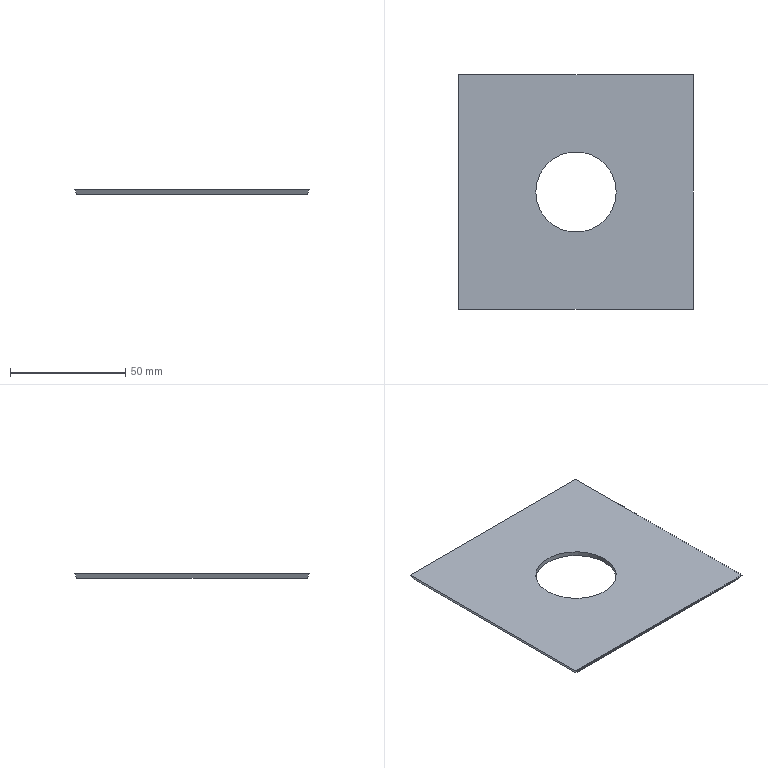Part | SolidWorks | features ICE 3, DeleteBody 2, Split 2, Blend 1, Shell 1 | 1 solid | 8 faces | box 102.046 x 102.046 x 2 mm | volume 18488 mm3 | plane 6 | cylinder 2 | commonest cylinder face diameters 35 x2
STEP:
#1=CARTESIAN_POINT('',(-17.5,0.,-350.));
#2=VERTEX_POINT('',#1);
#3=CARTESIAN_POINT('',(17.5,0.,-350.));
#4=VERTEX_POINT('',#3);
#5=CARTESIAN_POINT('',(0.,0.,-350.));
#6=DIRECTION('',(0.,0.,1.));
#7=DIRECTION('',(1.,0.,0.));
#8=AXIS2_PLACEMENT_3D('',#5,#6,#7);
#9=CIRCLE('',#8,17.5);
#10=EDGE_CURVE('',#2,#4,#9,.T.);
#11=ORIENTED_EDGE('',*,*,#10,.F.);
#12=CARTESIAN_POINT('',(-17.5,0.,-348.));
#13=VERTEX_POINT('',#12);
#14=CARTESIAN_POINT('',(-17.5,0.,-350.));
#15=DIRECTION('',(0.,0.,1.));
#16=VECTOR('',#15,1000.);
#17=LINE('',#14,#16);
#18=EDGE_CURVE('',#2,#13,#17,.T.);
#19=ORIENTED_EDGE('',*,*,#18,.T.);
#20=CARTESIAN_POINT('',(17.5,0.,-348.));
#21=VERTEX_POINT('',#20);
#22=CARTESIAN_POINT('',(0.,0.,-348.));
#23=DIRECTION('',(0.,0.,1.));
#24=DIRECTION('',(1.,0.,0.));
#25=AXIS2_PLACEMENT_3D('',#22,#23,#24);
#26=CIRCLE('',#25,17.5);
#27=EDGE_CURVE('',#13,#21,#26,.T.);
#28=ORIENTED_EDGE('',*,*,#27,.T.);
#29=CARTESIAN_POINT('',(17.5,0.,-350.));
#30=DIRECTION('',(0.,0.,1.));
#31=VECTOR('',#30,1000.);
#32=LINE('',#29,#31);
#33=EDGE_CURVE('',#4,#21,#32,.T.);
#34=ORIENTED_EDGE('',*,*,#33,.F.);
#35=EDGE_LOOP('',(#11,#19,#28,#34));
#36=FACE_OUTER_BOUND('',#35,.T.);
#37=CARTESIAN_POINT('',(0.,0.,-350.));
#38=DIRECTION('',(0.,0.,1.));
#39=DIRECTION('',(1.,0.,0.));
#40=AXIS2_PLACEMENT_3D('',#37,#38,#39);
#41=CYLINDRICAL_SURFACE('',#40,17.5);
#42=ADVANCED_FACE('',(#36),#41,.F.);
#43=CARTESIAN_POINT('',(-51.023,51.023,-348.));
#44=VERTEX_POINT('',#43);
#45=CARTESIAN_POINT('',(-50.,50.,-350.));
#46=VERTEX_POINT('',#45);
#47=CARTESIAN_POINT('',(-229.,229.,0.));
#48=DIRECTION('',(0.4144,-0.4144,-0.8103));
#49=VECTOR('',#48,1000.);
#50=LINE('',#47,#49);
#51=EDGE_CURVE('',#44,#46,#50,.T.);
#52=ORIENTED_EDGE('',*,*,#51,.F.);
#53=CARTESIAN_POINT('',(51.023,51.023,-348.));
#54=VERTEX_POINT('',#53);
#55=CARTESIAN_POINT('',(0.,51.023,-348.));
#56=DIRECTION('',(1.,0.,0.));
#57=VECTOR('',#56,1000.);
#58=LINE('',#55,#57);
#59=EDGE_CURVE('',#44,#54,#58,.T.);
#60=ORIENTED_EDGE('',*,*,#59,.T.);
#61=CARTESIAN_POINT('',(50.,50.,-350.));
#62=VERTEX_POINT('',#61);
#63=CARTESIAN_POINT('',(229.,229.,0.));
#64=DIRECTION('',(-0.4144,-0.4144,-0.8103));
#65=VECTOR('',#64,1000.);
#66=LINE('',#63,#65);
#67=EDGE_CURVE('',#54,#62,#66,.T.);
#68=ORIENTED_EDGE('',*,*,#67,.T.);
#69=CARTESIAN_POINT('',(-50.,50.,-350.));
#70=DIRECTION('',(-1.,0.,0.));
#71=VECTOR('',#70,1000.);
#72=LINE('',#69,#71);
#73=EDGE_CURVE('',#62,#46,#72,.T.);
#74=ORIENTED_EDGE('',*,*,#73,.T.);
#75=EDGE_LOOP('',(#52,#60,#68,#74));
#76=FACE_OUTER_BOUND('',#75,.T.);
#77=CARTESIAN_POINT('',(0.,181.521,-92.835));
#78=DIRECTION('',(0.,0.8903,-0.4553));
#79=DIRECTION('',(0.,0.4553,0.8903));
#80=AXIS2_PLACEMENT_3D('',#77,#78,#79);
#81=PLANE('',#80);
#82=ADVANCED_FACE('',(#76),#81,.T.);
#83=CARTESIAN_POINT('',(-51.023,-51.023,-348.));
#84=VERTEX_POINT('',#83);
#85=CARTESIAN_POINT('',(-50.,-50.,-350.));
#86=VERTEX_POINT('',#85);
#87=CARTESIAN_POINT('',(-229.,-229.,0.));
#88=DIRECTION('',(0.4144,0.4144,-0.8103));
#89=VECTOR('',#88,1000.);
#90=LINE('',#87,#89);
#91=EDGE_CURVE('',#84,#86,#90,.T.);
#92=ORIENTED_EDGE('',*,*,#91,.F.);
#93=CARTESIAN_POINT('',(-51.023,0.,-348.));
#94=DIRECTION('',(0.,1.,0.));
#95=VECTOR('',#94,1000.);
#96=LINE('',#93,#95);
#97=EDGE_CURVE('',#84,#44,#96,.T.);
#98=ORIENTED_EDGE('',*,*,#97,.T.);
#99=ORIENTED_EDGE('',*,*,#51,.T.);
#100=CARTESIAN_POINT('',(-50.,50.,-350.));
#101=DIRECTION('',(0.,-1.,0.));
#102=VECTOR('',#101,1000.);
#103=LINE('',#100,#102);
#104=EDGE_CURVE('',#46,#86,#103,.T.);
#105=ORIENTED_EDGE('',*,*,#104,.T.);
#106=EDGE_LOOP('',(#92,#98,#99,#105));
#107=FACE_OUTER_BOUND('',#106,.T.);
#108=CARTESIAN_POINT('',(-181.521,0.,-92.835));
#109=DIRECTION('',(-0.8903,0.,-0.4553));
#110=DIRECTION('',(-0.4553,0.,0.8903));
#111=AXIS2_PLACEMENT_3D('',#108,#109,#110);
#112=PLANE('',#111);
#113=ADVANCED_FACE('',(#107),#112,.T.);
#114=ORIENTED_EDGE('',*,*,#59,.F.);
#115=ORIENTED_EDGE('',*,*,#97,.F.);
#116=CARTESIAN_POINT('',(51.023,-51.023,-348.));
#117=VERTEX_POINT('',#116);
#118=CARTESIAN_POINT('',(0.,-51.023,-348.));
#119=DIRECTION('',(-1.,0.,0.));
#120=VECTOR('',#119,1000.);
#121=LINE('',#118,#120);
#122=EDGE_CURVE('',#117,#84,#121,.T.);
#123=ORIENTED_EDGE('',*,*,#122,.F.);
#124=CARTESIAN_POINT('',(51.023,0.,-348.));
#125=DIRECTION('',(0.,-1.,0.));
#126=VECTOR('',#125,1000.);
#127=LINE('',#124,#126);
#128=EDGE_CURVE('',#54,#117,#127,.T.);
#129=ORIENTED_EDGE('',*,*,#128,.F.);
#130=EDGE_LOOP('',(#114,#115,#123,#129));
#131=FACE_OUTER_BOUND('',#130,.T.);
#132=CARTESIAN_POINT('',(0.,0.,-348.));
#133=DIRECTION('',(0.,0.,1.));
#134=DIRECTION('',(1.,0.,0.));
#135=AXIS2_PLACEMENT_3D('',#132,#133,#134);
#136=CIRCLE('',#135,17.5);
#137=EDGE_CURVE('',#21,#13,#136,.T.);
#138=ORIENTED_EDGE('',*,*,#137,.F.);
#139=ORIENTED_EDGE('',*,*,#27,.F.);
#140=EDGE_LOOP('',(#138,#139));
#141=FACE_BOUND('',#140,.T.);
#142=CARTESIAN_POINT('',(48.776,48.776,-348.));
#143=DIRECTION('',(0.,0.,1.));
#144=DIRECTION('',(1.,0.,0.));
#145=AXIS2_PLACEMENT_3D('',#142,#143,#144);
#146=PLANE('',#145);
#147=ADVANCED_FACE('',(#131,#141),#146,.T.);
#148=ORIENTED_EDGE('',*,*,#67,.F.);
#149=ORIENTED_EDGE('',*,*,#128,.T.);
#150=CARTESIAN_POINT('',(50.,-50.,-350.));
#151=VERTEX_POINT('',#150);
#152=CARTESIAN_POINT('',(229.,-229.,0.));
#153=DIRECTION('',(-0.4144,0.4144,-0.8103));
#154=VECTOR('',#153,1000.);
#155=LINE('',#152,#154);
#156=EDGE_CURVE('',#117,#151,#155,.T.);
#157=ORIENTED_EDGE('',*,*,#156,.T.);
#158=CARTESIAN_POINT('',(50.,50.,-350.));
#159=DIRECTION('',(0.,1.,0.));
#160=VECTOR('',#159,1000.);
#161=LINE('',#158,#160);
#162=EDGE_CURVE('',#151,#62,#161,.T.);
#163=ORIENTED_EDGE('',*,*,#162,.T.);
#164=EDGE_LOOP('',(#148,#149,#157,#163));
#165=FACE_OUTER_BOUND('',#164,.T.);
#166=CARTESIAN_POINT('',(181.521,0.,-92.835));
#167=DIRECTION('',(0.8903,0.,-0.4553));
#168=DIRECTION('',(-0.4553,0.,-0.8903));
#169=AXIS2_PLACEMENT_3D('',#166,#167,#168);
#170=PLANE('',#169);
#171=ADVANCED_FACE('',(#165),#170,.T.);
#172=ORIENTED_EDGE('',*,*,#156,.F.);
#173=ORIENTED_EDGE('',*,*,#122,.T.);
#174=ORIENTED_EDGE('',*,*,#91,.T.);
#175=CARTESIAN_POINT('',(-50.,-50.,-350.));
#176=DIRECTION('',(1.,0.,0.));
#177=VECTOR('',#176,1000.);
#178=LINE('',#175,#177);
#179=EDGE_CURVE('',#86,#151,#178,.T.);
#180=ORIENTED_EDGE('',*,*,#179,.T.);
#181=EDGE_LOOP('',(#172,#173,#174,#180));
#182=FACE_OUTER_BOUND('',#181,.T.);
#183=CARTESIAN_POINT('',(0.,-181.521,-92.835));
#184=DIRECTION('',(0.,-0.8903,-0.4553));
#185=DIRECTION('',(0.,0.4553,-0.8903));
#186=AXIS2_PLACEMENT_3D('',#183,#184,#185);
#187=PLANE('',#186);
#188=ADVANCED_FACE('',(#182),#187,.T.);
#189=ORIENTED_EDGE('',*,*,#18,.F.);
#190=CARTESIAN_POINT('',(0.,0.,-350.));
#191=DIRECTION('',(0.,0.,1.));
#192=DIRECTION('',(1.,0.,0.));
#193=AXIS2_PLACEMENT_3D('',#190,#191,#192);
#194=CIRCLE('',#193,17.5);
#195=EDGE_CURVE('',#4,#2,#194,.T.);
#196=ORIENTED_EDGE('',*,*,#195,.F.);
#197=ORIENTED_EDGE('',*,*,#33,.T.);
#198=ORIENTED_EDGE('',*,*,#137,.T.);
#199=EDGE_LOOP('',(#189,#196,#197,#198));
#200=FACE_OUTER_BOUND('',#199,.T.);
#201=CARTESIAN_POINT('',(0.,0.,-350.));
#202=DIRECTION('',(0.,0.,1.));
#203=DIRECTION('',(1.,0.,0.));
#204=AXIS2_PLACEMENT_3D('',#201,#202,#203);
#205=CYLINDRICAL_SURFACE('',#204,17.5);
#206=ADVANCED_FACE('',(#200),#205,.F.);
#207=ORIENTED_EDGE('',*,*,#162,.F.);
#208=ORIENTED_EDGE('',*,*,#179,.F.);
#209=ORIENTED_EDGE('',*,*,#104,.F.);
#210=ORIENTED_EDGE('',*,*,#73,.F.);
#211=EDGE_LOOP('',(#207,#208,#209,#210));
#212=FACE_OUTER_BOUND('',#211,.T.);
#213=ORIENTED_EDGE('',*,*,#195,.T.);
#214=ORIENTED_EDGE('',*,*,#10,.T.);
#215=EDGE_LOOP('',(#213,#214));
#216=FACE_BOUND('',#215,.T.);
#217=CARTESIAN_POINT('',(50.,-50.,-350.));
#218=DIRECTION('',(0.,0.,-1.));
#219=DIRECTION('',(-1.,0.,0.));
#220=AXIS2_PLACEMENT_3D('',#217,#218,#219);
#221=PLANE('',#220);
#222=ADVANCED_FACE('',(#212,#216),#221,.T.);
#223=CLOSED_SHELL('',(#42,#82,#113,#147,#171,#188,#206,#222));
#224=MANIFOLD_SOLID_BREP('',#223);
#225=CARTESIAN_POINT('',(0.,0.,0.));
#226=DIRECTION('',(0.,0.,1.));
#227=DIRECTION('',(1.,0.,0.));
#228=AXIS2_PLACEMENT_3D('',#225,#226,#227);
#229=(LENGTH_UNIT()NAMED_UNIT(*)SI_UNIT(.MILLI.,.METRE.));
#230=UNCERTAINTY_MEASURE_WITH_UNIT(LENGTH_MEASURE(0.00001),#229,'','');
#231=(NAMED_UNIT(*)PLANE_ANGLE_UNIT()SI_UNIT($,.RADIAN.));
#232=(NAMED_UNIT(*)SI_UNIT($,.STERADIAN.)SOLID_ANGLE_UNIT());
#233=(GEOMETRIC_REPRESENTATION_CONTEXT(3)GLOBAL_UNCERTAINTY_ASSIGNED_CONTEXT((#230))GLOBAL_UNIT_ASSIGNED_CONTEXT((#229,#231,#232))REPRESENTATION_CONTEXT('',''));
#234=ADVANCED_BREP_SHAPE_REPRESENTATION('',(#224,#228),#233);